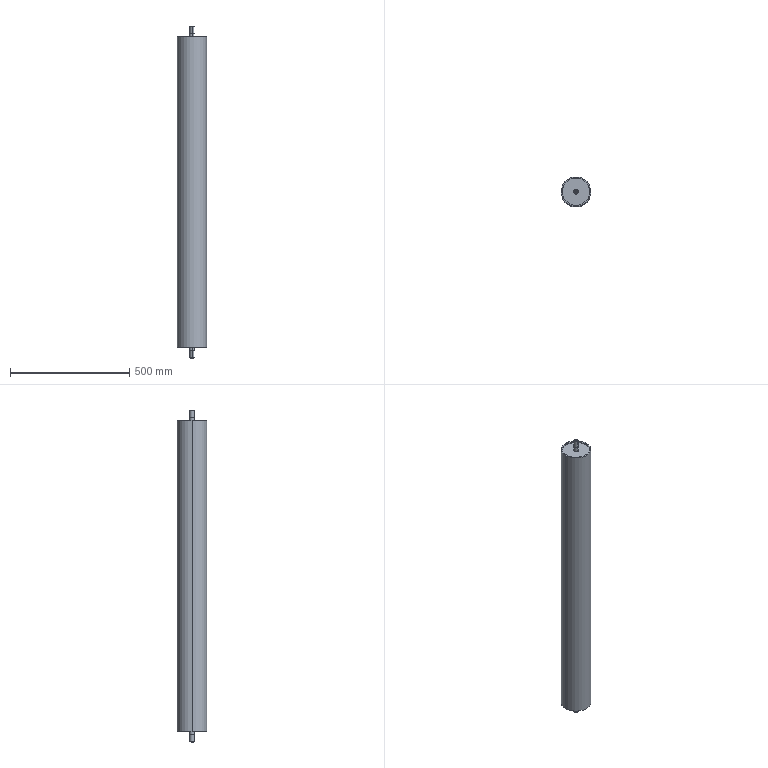Part | STEP file | Produce dryer-Driven part | 1 solid | 44 faces | box 124 x 124 x 1393 mm | volume 2869767 mm3 | cylinder 22 | cone 12 | plane 10 | commonest cylinder face diameters 20 x6 114.4 x6 5 x4 17 x4 124 x2
STEP:
#1=CARTESIAN_POINT('',(2.5,0.,-681.5));
#2=VERTEX_POINT('',#1);
#3=CARTESIAN_POINT('',(-2.5,0.,-681.5));
#4=VERTEX_POINT('',#3);
#5=CARTESIAN_POINT('',(0.,0.,-681.5));
#6=DIRECTION('',(0.,0.,-1.));
#7=DIRECTION('',(-1.,0.,0.));
#8=AXIS2_PLACEMENT_3D('',#5,#6,#7);
#9=CIRCLE('',#8,2.5);
#10=EDGE_CURVE('',#2,#4,#9,.T.);
#11=ORIENTED_EDGE('',*,*,#10,.F.);
#12=CARTESIAN_POINT('',(2.5,0.,-696.5));
#13=VERTEX_POINT('',#12);
#14=CARTESIAN_POINT('',(2.5,0.,-696.5));
#15=DIRECTION('',(0.,0.,-1.));
#16=VECTOR('',#15,1000.);
#17=LINE('',#14,#16);
#18=EDGE_CURVE('',#2,#13,#17,.T.);
#19=ORIENTED_EDGE('',*,*,#18,.T.);
#20=CARTESIAN_POINT('',(-2.5,0.,-696.5));
#21=VERTEX_POINT('',#20);
#22=CARTESIAN_POINT('',(0.,0.,-696.5));
#23=DIRECTION('',(0.,0.,-1.));
#24=DIRECTION('',(-1.,0.,0.));
#25=AXIS2_PLACEMENT_3D('',#22,#23,#24);
#26=CIRCLE('',#25,2.5);
#27=EDGE_CURVE('',#13,#21,#26,.T.);
#28=ORIENTED_EDGE('',*,*,#27,.T.);
#29=CARTESIAN_POINT('',(-2.5,0.,-696.5));
#30=DIRECTION('',(0.,0.,-1.));
#31=VECTOR('',#30,1000.);
#32=LINE('',#29,#31);
#33=EDGE_CURVE('',#4,#21,#32,.T.);
#34=ORIENTED_EDGE('',*,*,#33,.F.);
#35=EDGE_LOOP('',(#11,#19,#28,#34));
#36=FACE_OUTER_BOUND('',#35,.T.);
#37=CARTESIAN_POINT('',(0.,0.,-696.5));
#38=DIRECTION('',(0.,0.,-1.));
#39=DIRECTION('',(-1.,0.,0.));
#40=AXIS2_PLACEMENT_3D('',#37,#38,#39);
#41=CYLINDRICAL_SURFACE('',#40,2.5);
#42=ADVANCED_FACE('',(#36),#41,.F.);
#43=CARTESIAN_POINT('',(0.,0.,-679.998));
#44=VERTEX_POINT('',#43);
#45=CARTESIAN_POINT('',(-2.5,0.,-681.5));
#46=DIRECTION('',(-0.8572,0.,-0.515));
#47=VECTOR('',#46,1000.);
#48=LINE('',#45,#47);
#49=EDGE_CURVE('',#44,#4,#48,.T.);
#50=ORIENTED_EDGE('',*,*,#49,.F.);
#51=CARTESIAN_POINT('',(2.5,0.,-681.5));
#52=DIRECTION('',(0.8572,0.,-0.515));
#53=VECTOR('',#52,1000.);
#54=LINE('',#51,#53);
#55=EDGE_CURVE('',#44,#2,#54,.T.);
#56=ORIENTED_EDGE('',*,*,#55,.T.);
#57=ORIENTED_EDGE('',*,*,#10,.T.);
#58=EDGE_LOOP('',(#50,#56,#57));
#59=FACE_OUTER_BOUND('',#58,.T.);
#60=CARTESIAN_POINT('',(0.,0.,-681.5));
#61=DIRECTION('',(0.,0.,-1.));
#62=DIRECTION('',(-1.,0.,0.));
#63=AXIS2_PLACEMENT_3D('',#60,#61,#62);
#64=CONICAL_SURFACE('',#63,2.5,1.03);
#65=ADVANCED_FACE('',(#59),#64,.F.);
#66=CARTESIAN_POINT('',(0.,-10.,-665.));
#67=VERTEX_POINT('',#66);
#68=CARTESIAN_POINT('',(0.,10.,-665.));
#69=VERTEX_POINT('',#68);
#70=CARTESIAN_POINT('',(0.,0.,-665.));
#71=DIRECTION('',(0.,0.,1.));
#72=DIRECTION('',(0.,-1.,0.));
#73=AXIS2_PLACEMENT_3D('',#70,#71,#72);
#74=CIRCLE('',#73,10.);
#75=EDGE_CURVE('',#67,#69,#74,.T.);
#76=ORIENTED_EDGE('',*,*,#75,.T.);
#77=CARTESIAN_POINT('',(0.,10.,-645.5));
#78=VERTEX_POINT('',#77);
#79=CARTESIAN_POINT('',(0.,10.,-696.5));
#80=DIRECTION('',(0.,0.,1.));
#81=VECTOR('',#80,1000.);
#82=LINE('',#79,#81);
#83=EDGE_CURVE('',#69,#78,#82,.T.);
#84=ORIENTED_EDGE('',*,*,#83,.T.);
#85=CARTESIAN_POINT('',(0.,-10.,-645.5));
#86=VERTEX_POINT('',#85);
#87=CARTESIAN_POINT('',(0.,0.,-645.5));
#88=DIRECTION('',(0.,0.,-1.));
#89=DIRECTION('',(-1.,0.,0.));
#90=AXIS2_PLACEMENT_3D('',#87,#88,#89);
#91=CIRCLE('',#90,10.);
#92=EDGE_CURVE('',#78,#86,#91,.T.);
#93=ORIENTED_EDGE('',*,*,#92,.T.);
#94=CARTESIAN_POINT('',(0.,-10.,-696.5));
#95=DIRECTION('',(0.,0.,1.));
#96=VECTOR('',#95,1000.);
#97=LINE('',#94,#96);
#98=EDGE_CURVE('',#67,#86,#97,.T.);
#99=ORIENTED_EDGE('',*,*,#98,.F.);
#100=EDGE_LOOP('',(#76,#84,#93,#99));
#101=FACE_OUTER_BOUND('',#100,.T.);
#102=CARTESIAN_POINT('',(0.,0.,-696.5));
#103=DIRECTION('',(0.,0.,1.));
#104=DIRECTION('',(0.,-1.,0.));
#105=AXIS2_PLACEMENT_3D('',#102,#103,#104);
#106=CYLINDRICAL_SURFACE('',#105,10.);
#107=ADVANCED_FACE('',(#101),#106,.T.);
#108=CARTESIAN_POINT('',(0.,9.5,-665.5));
#109=VERTEX_POINT('',#108);
#110=CARTESIAN_POINT('',(0.,-9.5,-665.5));
#111=VERTEX_POINT('',#110);
#112=CARTESIAN_POINT('',(0.,0.,-665.5));
#113=DIRECTION('',(0.,0.,-1.));
#114=DIRECTION('',(0.,-1.,0.));
#115=AXIS2_PLACEMENT_3D('',#112,#113,#114);
#116=CIRCLE('',#115,9.5);
#117=EDGE_CURVE('',#109,#111,#116,.T.);
#118=ORIENTED_EDGE('',*,*,#117,.F.);
#119=CARTESIAN_POINT('',(0.,10.,-665.));
#120=DIRECTION('',(0.,0.7071,0.7071));
#121=VECTOR('',#120,1000.);
#122=LINE('',#119,#121);
#123=EDGE_CURVE('',#109,#69,#122,.T.);
#124=ORIENTED_EDGE('',*,*,#123,.T.);
#125=ORIENTED_EDGE('',*,*,#75,.F.);
#126=CARTESIAN_POINT('',(0.,-10.,-665.));
#127=DIRECTION('',(0.,-0.7071,0.7071));
#128=VECTOR('',#127,1000.);
#129=LINE('',#126,#128);
#130=EDGE_CURVE('',#111,#67,#129,.T.);
#131=ORIENTED_EDGE('',*,*,#130,.F.);
#132=EDGE_LOOP('',(#118,#124,#125,#131));
#133=FACE_OUTER_BOUND('',#132,.T.);
#134=CARTESIAN_POINT('',(0.,0.,-665.));
#135=DIRECTION('',(0.,0.,1.));
#136=DIRECTION('',(0.,-1.,0.));
#137=AXIS2_PLACEMENT_3D('',#134,#135,#136);
#138=CONICAL_SURFACE('',#137,10.,0.7854);
#139=ADVANCED_FACE('',(#133),#138,.T.);
#140=CARTESIAN_POINT('',(0.,-8.5,-696.));
#141=VERTEX_POINT('',#140);
#142=CARTESIAN_POINT('',(0.,8.5,-696.));
#143=VERTEX_POINT('',#142);
#144=CARTESIAN_POINT('',(0.,0.,-696.));
#145=DIRECTION('',(0.,0.,1.));
#146=DIRECTION('',(0.,-1.,0.));
#147=AXIS2_PLACEMENT_3D('',#144,#145,#146);
#148=CIRCLE('',#147,8.5);
#149=EDGE_CURVE('',#141,#143,#148,.T.);
#150=ORIENTED_EDGE('',*,*,#149,.T.);
#151=CARTESIAN_POINT('',(0.,8.5,-665.5));
#152=VERTEX_POINT('',#151);
#153=CARTESIAN_POINT('',(0.,8.5,-696.5));
#154=DIRECTION('',(0.,0.,1.));
#155=VECTOR('',#154,1000.);
#156=LINE('',#153,#155);
#157=EDGE_CURVE('',#143,#152,#156,.T.);
#158=ORIENTED_EDGE('',*,*,#157,.T.);
#159=CARTESIAN_POINT('',(0.,-8.5,-665.5));
#160=VERTEX_POINT('',#159);
#161=CARTESIAN_POINT('',(0.,0.,-665.5));
#162=DIRECTION('',(0.,0.,1.));
#163=DIRECTION('',(0.,-1.,0.));
#164=AXIS2_PLACEMENT_3D('',#161,#162,#163);
#165=CIRCLE('',#164,8.5);
#166=EDGE_CURVE('',#160,#152,#165,.T.);
#167=ORIENTED_EDGE('',*,*,#166,.F.);
#168=CARTESIAN_POINT('',(0.,-8.5,-696.5));
#169=DIRECTION('',(0.,0.,1.));
#170=VECTOR('',#169,1000.);
#171=LINE('',#168,#170);
#172=EDGE_CURVE('',#141,#160,#171,.T.);
#173=ORIENTED_EDGE('',*,*,#172,.F.);
#174=EDGE_LOOP('',(#150,#158,#167,#173));
#175=FACE_OUTER_BOUND('',#174,.T.);
#176=CARTESIAN_POINT('',(0.,0.,-696.5));
#177=DIRECTION('',(0.,0.,1.));
#178=DIRECTION('',(0.,-1.,0.));
#179=AXIS2_PLACEMENT_3D('',#176,#177,#178);
#180=CYLINDRICAL_SURFACE('',#179,8.5);
#181=ADVANCED_FACE('',(#175),#180,.T.);
#182=CARTESIAN_POINT('',(0.,8.,-696.5));
#183=VERTEX_POINT('',#182);
#184=CARTESIAN_POINT('',(0.,-8.,-696.5));
#185=VERTEX_POINT('',#184);
#186=CARTESIAN_POINT('',(0.,0.,-696.5));
#187=DIRECTION('',(0.,0.,-1.));
#188=DIRECTION('',(0.,-1.,0.));
#189=AXIS2_PLACEMENT_3D('',#186,#187,#188);
#190=CIRCLE('',#189,8.);
#191=EDGE_CURVE('',#183,#185,#190,.T.);
#192=ORIENTED_EDGE('',*,*,#191,.F.);
#193=CARTESIAN_POINT('',(0.,8.5,-696.));
#194=DIRECTION('',(0.,0.7071,0.7071));
#195=VECTOR('',#194,1000.);
#196=LINE('',#193,#195);
#197=EDGE_CURVE('',#183,#143,#196,.T.);
#198=ORIENTED_EDGE('',*,*,#197,.T.);
#199=ORIENTED_EDGE('',*,*,#149,.F.);
#200=CARTESIAN_POINT('',(0.,-8.5,-696.));
#201=DIRECTION('',(0.,-0.7071,0.7071));
#202=VECTOR('',#201,1000.);
#203=LINE('',#200,#202);
#204=EDGE_CURVE('',#185,#141,#203,.T.);
#205=ORIENTED_EDGE('',*,*,#204,.F.);
#206=EDGE_LOOP('',(#192,#198,#199,#205));
#207=FACE_OUTER_BOUND('',#206,.T.);
#208=CARTESIAN_POINT('',(0.,0.,-696.));
#209=DIRECTION('',(0.,0.,1.));
#210=DIRECTION('',(0.,-1.,0.));
#211=AXIS2_PLACEMENT_3D('',#208,#209,#210);
#212=CONICAL_SURFACE('',#211,8.5,0.7854);
#213=ADVANCED_FACE('',(#207),#212,.T.);
#214=CARTESIAN_POINT('',(-2.5,0.,681.5));
#215=VERTEX_POINT('',#214);
#216=CARTESIAN_POINT('',(2.5,0.,681.5));
#217=VERTEX_POINT('',#216);
#218=CARTESIAN_POINT('',(0.,0.,681.5));
#219=DIRECTION('',(0.,0.,1.));
#220=DIRECTION('',(1.,0.,0.));
#221=AXIS2_PLACEMENT_3D('',#218,#219,#220);
#222=CIRCLE('',#221,2.5);
#223=EDGE_CURVE('',#215,#217,#222,.T.);
#224=ORIENTED_EDGE('',*,*,#223,.F.);
#225=CARTESIAN_POINT('',(-2.5,0.,696.5));
#226=VERTEX_POINT('',#225);
#227=CARTESIAN_POINT('',(-2.5,0.,696.5));
#228=DIRECTION('',(0.,0.,1.));
#229=VECTOR('',#228,1000.);
#230=LINE('',#227,#229);
#231=EDGE_CURVE('',#215,#226,#230,.T.);
#232=ORIENTED_EDGE('',*,*,#231,.T.);
#233=CARTESIAN_POINT('',(2.5,0.,696.5));
#234=VERTEX_POINT('',#233);
#235=CARTESIAN_POINT('',(0.,0.,696.5));
#236=DIRECTION('',(0.,0.,1.));
#237=DIRECTION('',(1.,0.,0.));
#238=AXIS2_PLACEMENT_3D('',#235,#236,#237);
#239=CIRCLE('',#238,2.5);
#240=EDGE_CURVE('',#226,#234,#239,.T.);
#241=ORIENTED_EDGE('',*,*,#240,.T.);
#242=CARTESIAN_POINT('',(2.5,0.,696.5));
#243=DIRECTION('',(0.,0.,1.));
#244=VECTOR('',#243,1000.);
#245=LINE('',#242,#244);
#246=EDGE_CURVE('',#217,#234,#245,.T.);
#247=ORIENTED_EDGE('',*,*,#246,.F.);
#248=EDGE_LOOP('',(#224,#232,#241,#247));
#249=FACE_OUTER_BOUND('',#248,.T.);
#250=CARTESIAN_POINT('',(0.,0.,696.5));
#251=DIRECTION('',(0.,0.,1.));
#252=DIRECTION('',(1.,0.,0.));
#253=AXIS2_PLACEMENT_3D('',#250,#251,#252);
#254=CYLINDRICAL_SURFACE('',#253,2.5);
#255=ADVANCED_FACE('',(#249),#254,.F.);
#256=CARTESIAN_POINT('',(0.,0.,679.998));
#257=VERTEX_POINT('',#256);
#258=CARTESIAN_POINT('',(2.5,0.,681.5));
#259=DIRECTION('',(0.8572,0.,0.515));
#260=VECTOR('',#259,1000.);
#261=LINE('',#258,#260);
#262=EDGE_CURVE('',#257,#217,#261,.T.);
#263=ORIENTED_EDGE('',*,*,#262,.F.);
#264=CARTESIAN_POINT('',(-2.5,0.,681.5));
#265=DIRECTION('',(-0.8572,0.,0.515));
#266=VECTOR('',#265,1000.);
#267=LINE('',#264,#266);
#268=EDGE_CURVE('',#257,#215,#267,.T.);
#269=ORIENTED_EDGE('',*,*,#268,.T.);
#270=ORIENTED_EDGE('',*,*,#223,.T.);
#271=EDGE_LOOP('',(#263,#269,#270));
#272=FACE_OUTER_BOUND('',#271,.T.);
#273=CARTESIAN_POINT('',(0.,0.,681.5));
#274=DIRECTION('',(0.,0.,1.));
#275=DIRECTION('',(1.,0.,0.));
#276=AXIS2_PLACEMENT_3D('',#273,#274,#275);
#277=CONICAL_SURFACE('',#276,2.5,1.03);
#278=ADVANCED_FACE('',(#272),#277,.F.);
#279=CARTESIAN_POINT('',(0.,-9.5,665.5));
#280=VERTEX_POINT('',#279);
#281=CARTESIAN_POINT('',(0.,9.5,665.5));
#282=VERTEX_POINT('',#281);
#283=CARTESIAN_POINT('',(0.,0.,665.5));
#284=DIRECTION('',(0.,0.,1.));
#285=DIRECTION('',(0.,1.,0.));
#286=AXIS2_PLACEMENT_3D('',#283,#284,#285);
#287=CIRCLE('',#286,9.5);
#288=EDGE_CURVE('',#280,#282,#287,.T.);
#289=ORIENTED_EDGE('',*,*,#288,.F.);
#290=CARTESIAN_POINT('',(0.,-10.,665.));
#291=VERTEX_POINT('',#290);
#292=CARTESIAN_POINT('',(0.,-9.5,665.5));
#293=DIRECTION('',(0.,-0.7071,-0.7071));
#294=VECTOR('',#293,1000.);
#295=LINE('',#292,#294);
#296=EDGE_CURVE('',#280,#291,#295,.T.);
#297=ORIENTED_EDGE('',*,*,#296,.T.);
#298=CARTESIAN_POINT('',(0.,10.,665.));
#299=VERTEX_POINT('',#298);
#300=CARTESIAN_POINT('',(0.,0.,665.));
#301=DIRECTION('',(0.,0.,-1.));
#302=DIRECTION('',(0.,1.,0.));
#303=AXIS2_PLACEMENT_3D('',#300,#301,#302);
#304=CIRCLE('',#303,10.);
#305=EDGE_CURVE('',#299,#291,#304,.T.);
#306=ORIENTED_EDGE('',*,*,#305,.F.);
#307=CARTESIAN_POINT('',(0.,9.5,665.5));
#308=DIRECTION('',(0.,0.7071,-0.7071));
#309=VECTOR('',#308,1000.);
#310=LINE('',#307,#309);
#311=EDGE_CURVE('',#282,#299,#310,.T.);
#312=ORIENTED_EDGE('',*,*,#311,.F.);
#313=EDGE_LOOP('',(#289,#297,#306,#312));
#314=FACE_OUTER_BOUND('',#313,.T.);
#315=CARTESIAN_POINT('',(0.,0.,665.5));
#316=DIRECTION('',(0.,0.,-1.));
#317=DIRECTION('',(0.,1.,0.));
#318=AXIS2_PLACEMENT_3D('',#315,#316,#317);
#319=CONICAL_SURFACE('',#318,9.5,0.7854);
#320=ADVANCED_FACE('',(#314),#319,.T.);
#321=CARTESIAN_POINT('',(0.,-8.,696.5));
#322=VERTEX_POINT('',#321);
#323=CARTESIAN_POINT('',(0.,8.,696.5));
#324=VERTEX_POINT('',#323);
#325=CARTESIAN_POINT('',(0.,0.,696.5));
#326=DIRECTION('',(0.,0.,1.));
#327=DIRECTION('',(0.,1.,0.));
#328=AXIS2_PLACEMENT_3D('',#325,#326,#327);
#329=CIRCLE('',#328,8.);
#330=EDGE_CURVE('',#322,#324,#329,.T.);
#331=ORIENTED_EDGE('',*,*,#330,.F.);
#332=CARTESIAN_POINT('',(0.,-8.5,696.));
#333=VERTEX_POINT('',#332);
#334=CARTESIAN_POINT('',(0.,-8.,696.5));
#335=DIRECTION('',(0.,-0.7071,-0.7071));
#336=VECTOR('',#335,1000.);
#337=LINE('',#334,#336);
#338=EDGE_CURVE('',#322,#333,#337,.T.);
#339=ORIENTED_EDGE('',*,*,#338,.T.);
#340=CARTESIAN_POINT('',(0.,8.5,696.));
#341=VERTEX_POINT('',#340);
#342=CARTESIAN_POINT('',(0.,0.,696.));
#343=DIRECTION('',(0.,0.,-1.));
#344=DIRECTION('',(0.,1.,0.));
#345=AXIS2_PLACEMENT_3D('',#342,#343,#344);
#346=CIRCLE('',#345,8.5);
#347=EDGE_CURVE('',#341,#333,#346,.T.);
#348=ORIENTED_EDGE('',*,*,#347,.F.);
#349=CARTESIAN_POINT('',(0.,8.,696.5));
#350=DIRECTION('',(0.,0.7071,-0.7071));
#351=VECTOR('',#350,1000.);
#352=LINE('',#349,#351);
#353=EDGE_CURVE('',#324,#341,#352,.T.);
#354=ORIENTED_EDGE('',*,*,#353,.F.);
#355=EDGE_LOOP('',(#331,#339,#348,#354));
#356=FACE_OUTER_BOUND('',#355,.T.);
#357=CARTESIAN_POINT('',(0.,0.,696.5));
#358=DIRECTION('',(0.,0.,-1.));
#359=DIRECTION('',(0.,1.,0.));
#360=AXIS2_PLACEMENT_3D('',#357,#358,#359);
#361=CONICAL_SURFACE('',#360,8.,0.7854);
#362=ADVANCED_FACE('',(#356),#361,.T.);
#363=CARTESIAN_POINT('',(0.,10.,645.5));
#364=VERTEX_POINT('',#363);
#365=CARTESIAN_POINT('',(0.,-10.,645.5));
#366=VERTEX_POINT('',#365);
#367=CARTESIAN_POINT('',(0.,0.,645.5));
#368=DIRECTION('',(0.,0.,-1.));
#369=DIRECTION('',(1.,0.,0.));
#370=AXIS2_PLACEMENT_3D('',#367,#368,#369);
#371=CIRCLE('',#370,10.);
#372=EDGE_CURVE('',#364,#366,#371,.T.);
#373=ORIENTED_EDGE('',*,*,#372,.F.);
#374=CARTESIAN_POINT('',(0.,10.,-696.5));
#375=DIRECTION('',(0.,0.,1.));
#376=VECTOR('',#375,1000.);
#377=LINE('',#374,#376);
#378=EDGE_CURVE('',#364,#299,#377,.T.);
#379=ORIENTED_EDGE('',*,*,#378,.T.);
#380=ORIENTED_EDGE('',*,*,#305,.T.);
#381=CARTESIAN_POINT('',(0.,-10.,-696.5));
#382=DIRECTION('',(0.,0.,1.));
#383=VECTOR('',#382,1000.);
#384=LINE('',#381,#383);
#385=EDGE_CURVE('',#366,#291,#384,.T.);
#386=ORIENTED_EDGE('',*,*,#385,.F.);
#387=EDGE_LOOP('',(#373,#379,#380,#386));
#388=FACE_OUTER_BOUND('',#387,.T.);
#389=CARTESIAN_POINT('',(0.,0.,-696.5));
#390=DIRECTION('',(0.,0.,1.));
#391=DIRECTION('',(0.,-1.,0.));
#392=AXIS2_PLACEMENT_3D('',#389,#390,#391);
#393=CYLINDRICAL_SURFACE('',#392,10.);
#394=ADVANCED_FACE('',(#388),#393,.T.);
#395=CARTESIAN_POINT('',(0.,-8.5,665.5));
#396=VERTEX_POINT('',#395);
#397=CARTESIAN_POINT('',(0.,8.5,665.5));
#398=VERTEX_POINT('',#397);
#399=CARTESIAN_POINT('',(0.,0.,665.5));
#400=DIRECTION('',(0.,0.,1.));
#401=DIRECTION('',(0.,-1.,0.));
#402=AXIS2_PLACEMENT_3D('',#399,#400,#401);
#403=CIRCLE('',#402,8.5);
#404=EDGE_CURVE('',#396,#398,#403,.T.);
#405=ORIENTED_EDGE('',*,*,#404,.T.);
#406=CARTESIAN_POINT('',(0.,8.5,-696.5));
#407=DIRECTION('',(0.,0.,1.));
#408=VECTOR('',#407,1000.);
#409=LINE('',#406,#408);
#410=EDGE_CURVE('',#398,#341,#409,.T.);
#411=ORIENTED_EDGE('',*,*,#410,.T.);
#412=ORIENTED_EDGE('',*,*,#347,.T.);
#413=CARTESIAN_POINT('',(0.,-8.5,-696.5));
#414=DIRECTION('',(0.,0.,1.));
#415=VECTOR('',#414,1000.);
#416=LINE('',#413,#415);
#417=EDGE_CURVE('',#396,#333,#416,.T.);
#418=ORIENTED_EDGE('',*,*,#417,.F.);
#419=EDGE_LOOP('',(#405,#411,#412,#418));
#420=FACE_OUTER_BOUND('',#419,.T.);
#421=CARTESIAN_POINT('',(0.,0.,-696.5));
#422=DIRECTION('',(0.,0.,1.));
#423=DIRECTION('',(0.,-1.,0.));
#424=AXIS2_PLACEMENT_3D('',#421,#422,#423);
#425=CYLINDRICAL_SURFACE('',#424,8.5);
#426=ADVANCED_FACE('',(#420),#425,.T.);
#427=CARTESIAN_POINT('',(-57.2,0.,650.5));
#428=VERTEX_POINT('',#427);
#429=CARTESIAN_POINT('',(57.2,0.,650.5));
#430=VERTEX_POINT('',#429);
#431=CARTESIAN_POINT('',(0.,0.,650.5));
#432=DIRECTION('',(0.,0.,1.));
#433=DIRECTION('',(1.,0.,0.));
#434=AXIS2_PLACEMENT_3D('',#431,#432,#433);
#435=CIRCLE('',#434,57.2);
#436=EDGE_CURVE('',#428,#430,#435,.T.);
#437=ORIENTED_EDGE('',*,*,#436,.T.);
#438=CARTESIAN_POINT('',(57.2,0.,645.5));
#439=VERTEX_POINT('',#438);
#440=CARTESIAN_POINT('',(57.2,0.,650.5));
#441=DIRECTION('',(0.,0.,-1.));
#442=VECTOR('',#441,1000.);
#443=LINE('',#440,#442);
#444=EDGE_CURVE('',#430,#439,#443,.T.);
#445=ORIENTED_EDGE('',*,*,#444,.T.);
#446=CARTESIAN_POINT('',(-57.2,0.,645.5));
#447=VERTEX_POINT('',#446);
#448=CARTESIAN_POINT('',(0.,0.,645.5));
#449=DIRECTION('',(0.,0.,1.));
#450=DIRECTION('',(1.,0.,0.));
#451=AXIS2_PLACEMENT_3D('',#448,#449,#450);
#452=CIRCLE('',#451,57.2);
#453=EDGE_CURVE('',#447,#439,#452,.T.);
#454=ORIENTED_EDGE('',*,*,#453,.F.);
#455=CARTESIAN_POINT('',(-57.2,0.,650.5));
#456=DIRECTION('',(0.,0.,-1.));
#457=VECTOR('',#456,1000.);
#458=LINE('',#455,#457);
#459=EDGE_CURVE('',#428,#447,#458,.T.);
#460=ORIENTED_EDGE('',*,*,#459,.F.);
#461=EDGE_LOOP('',(#437,#445,#454,#460));
#462=FACE_OUTER_BOUND('',#461,.T.);
#463=CARTESIAN_POINT('',(0.,0.,650.5));
#464=DIRECTION('',(0.,0.,-1.));
#465=DIRECTION('',(-1.,0.,0.));
#466=AXIS2_PLACEMENT_3D('',#463,#464,#465);
#467=CYLINDRICAL_SURFACE('',#466,57.2);
#468=ADVANCED_FACE('',(#462),#467,.F.);
#469=CARTESIAN_POINT('',(62.,0.,650.5));
#470=VERTEX_POINT('',#469);
#471=CARTESIAN_POINT('',(-62.,0.,650.5));
#472=VERTEX_POINT('',#471);
#473=CARTESIAN_POINT('',(0.,0.,650.5));
#474=DIRECTION('',(0.,0.,1.));
#475=DIRECTION('',(1.,0.,0.));
#476=AXIS2_PLACEMENT_3D('',#473,#474,#475);
#477=CIRCLE('',#476,62.);
#478=EDGE_CURVE('',#470,#472,#477,.T.);
#479=ORIENTED_EDGE('',*,*,#478,.F.);
#480=CARTESIAN_POINT('',(62.,0.,-650.5));
#481=VERTEX_POINT('',#480);
#482=CARTESIAN_POINT('',(62.,0.,650.5));
#483=DIRECTION('',(0.,0.,-1.));
#484=VECTOR('',#483,1000.);
#485=LINE('',#482,#484);
#486=EDGE_CURVE('',#470,#481,#485,.T.);
#487=ORIENTED_EDGE('',*,*,#486,.T.);
#488=CARTESIAN_POINT('',(-62.,0.,-650.5));
#489=VERTEX_POINT('',#488);
#490=CARTESIAN_POINT('',(0.,0.,-650.5));
#491=DIRECTION('',(0.,0.,1.));
#492=DIRECTION('',(1.,0.,0.));
#493=AXIS2_PLACEMENT_3D('',#490,#491,#492);
#494=CIRCLE('',#493,62.);
#495=EDGE_CURVE('',#481,#489,#494,.T.);
#496=ORIENTED_EDGE('',*,*,#495,.T.);
#497=CARTESIAN_POINT('',(-62.,0.,650.5));
#498=DIRECTION('',(0.,0.,-1.));
#499=VECTOR('',#498,1000.);
#500=LINE('',#497,#499);
#501=EDGE_CURVE('',#472,#489,#500,.T.);
#502=ORIENTED_EDGE('',*,*,#501,.F.);
#503=EDGE_LOOP('',(#479,#487,#496,#502));
#504=FACE_OUTER_BOUND('',#503,.T.);
#505=CARTESIAN_POINT('',(0.,0.,650.5));
#506=DIRECTION('',(0.,0.,-1.));
#507=DIRECTION('',(-1.,0.,0.));
#508=AXIS2_PLACEMENT_3D('',#505,#506,#507);
#509=CYLINDRICAL_SURFACE('',#508,62.);
#510=ADVANCED_FACE('',(#504),#509,.T.);
#511=CARTESIAN_POINT('',(57.2,0.,-645.5));
#512=VERTEX_POINT('',#511);
#513=CARTESIAN_POINT('',(-57.2,0.,-645.5));
#514=VERTEX_POINT('',#513);
#515=CARTESIAN_POINT('',(0.,0.,-645.5));
#516=DIRECTION('',(0.,0.,-1.));
#517=DIRECTION('',(-1.,0.,0.));
#518=AXIS2_PLACEMENT_3D('',#515,#516,#517);
#519=CIRCLE('',#518,57.2);
#520=EDGE_CURVE('',#512,#514,#519,.T.);
#521=ORIENTED_EDGE('',*,*,#520,.F.);
#522=CARTESIAN_POINT('',(57.2,0.,-650.5));
#523=VERTEX_POINT('',#522);
#524=CARTESIAN_POINT('',(57.2,0.,650.5));
#525=DIRECTION('',(0.,0.,-1.));
#526=VECTOR('',#525,1000.);
#527=LINE('',#524,#526);
#528=EDGE_CURVE('',#512,#523,#527,.T.);
#529=ORIENTED_EDGE('',*,*,#528,.T.);
#530=CARTESIAN_POINT('',(-57.2,0.,-650.5));
#531=VERTEX_POINT('',#530);
#532=CARTESIAN_POINT('',(0.,0.,-650.5));
#533=DIRECTION('',(0.,0.,1.));
#534=DIRECTION('',(1.,0.,0.));
#535=AXIS2_PLACEMENT_3D('',#532,#533,#534);
#536=CIRCLE('',#535,57.2);
#537=EDGE_CURVE('',#531,#523,#536,.T.);
#538=ORIENTED_EDGE('',*,*,#537,.F.);
#539=CARTESIAN_POINT('',(-57.2,0.,650.5));
#540=DIRECTION('',(0.,0.,-1.));
#541=VECTOR('',#540,1000.);
#542=LINE('',#539,#541);
#543=EDGE_CURVE('',#514,#531,#542,.T.);
#544=ORIENTED_EDGE('',*,*,#543,.F.);
#545=EDGE_LOOP('',(#521,#529,#538,#544));
#546=FACE_OUTER_BOUND('',#545,.T.);
#547=CARTESIAN_POINT('',(0.,0.,650.5));
#548=DIRECTION('',(0.,0.,-1.));
#549=DIRECTION('',(-1.,0.,0.));
#550=AXIS2_PLACEMENT_3D('',#547,#548,#549);
#551=CYLINDRICAL_SURFACE('',#550,57.2);
#552=ADVANCED_FACE('',(#546),#551,.F.);
#553=ORIENTED_EDGE('',*,*,#528,.F.);
#554=CARTESIAN_POINT('',(0.,0.,-645.5));
#555=DIRECTION('',(0.,0.,-1.));
#556=DIRECTION('',(-1.,0.,0.));
#557=AXIS2_PLACEMENT_3D('',#554,#555,#556);
#558=CIRCLE('',#557,57.2);
#559=EDGE_CURVE('',#514,#512,#558,.T.);
#560=ORIENTED_EDGE('',*,*,#559,.F.);
#561=ORIENTED_EDGE('',*,*,#543,.T.);
#562=CARTESIAN_POINT('',(0.,0.,-650.5));
#563=DIRECTION('',(0.,0.,1.));
#564=DIRECTION('',(1.,0.,0.));
#565=AXIS2_PLACEMENT_3D('',#562,#563,#564);
#566=CIRCLE('',#565,57.2);
#567=EDGE_CURVE('',#523,#531,#566,.T.);
#568=ORIENTED_EDGE('',*,*,#567,.F.);
#569=EDGE_LOOP('',(#553,#560,#561,#568));
#570=FACE_OUTER_BOUND('',#569,.T.);
#571=CARTESIAN_POINT('',(0.,0.,650.5));
#572=DIRECTION('',(0.,0.,-1.));
#573=DIRECTION('',(-1.,0.,0.));
#574=AXIS2_PLACEMENT_3D('',#571,#572,#573);
#575=CYLINDRICAL_SURFACE('',#574,57.2);
#576=ADVANCED_FACE('',(#570),#575,.F.);
#577=CARTESIAN_POINT('',(0.,0.,650.5));
#578=DIRECTION('',(0.,0.,1.));
#579=DIRECTION('',(1.,0.,0.));
#580=AXIS2_PLACEMENT_3D('',#577,#578,#579);
#581=CIRCLE('',#580,62.);
#582=EDGE_CURVE('',#472,#470,#581,.T.);
#583=ORIENTED_EDGE('',*,*,#582,.T.);
#584=ORIENTED_EDGE('',*,*,#478,.T.);
#585=EDGE_LOOP('',(#583,#584));
#586=FACE_OUTER_BOUND('',#585,.T.);
#587=ORIENTED_EDGE('',*,*,#436,.F.);
#588=CARTESIAN_POINT('',(0.,0.,650.5));
#589=DIRECTION('',(0.,0.,1.));
#590=DIRECTION('',(1.,0.,0.));
#591=AXIS2_PLACEMENT_3D('',#588,#589,#590);
#592=CIRCLE('',#591,57.2);
#593=EDGE_CURVE('',#430,#428,#592,.T.);
#594=ORIENTED_EDGE('',*,*,#593,.F.);
#595=EDGE_LOOP('',(#587,#594));
#596=FACE_BOUND('',#595,.T.);
#597=CARTESIAN_POINT('',(0.,0.,650.5));
#598=DIRECTION('',(0.,0.,1.));
#599=DIRECTION('',(1.,0.,0.));
#600=AXIS2_PLACEMENT_3D('',#597,#598,#599);
#601=PLANE('',#600);
#602=ADVANCED_FACE('',(#586,#596),#601,.T.);
#603=CARTESIAN_POINT('',(0.,0.,-650.5));
#604=DIRECTION('',(0.,0.,1.));
#605=DIRECTION('',(1.,0.,0.));
#606=AXIS2_PLACEMENT_3D('',#603,#604,#605);
#607=CIRCLE('',#606,62.);
#608=EDGE_CURVE('',#489,#481,#607,.T.);
#609=ORIENTED_EDGE('',*,*,#608,.F.);
#610=ORIENTED_EDGE('',*,*,#495,.F.);
#611=EDGE_LOOP('',(#609,#610));
#612=FACE_OUTER_BOUND('',#611,.T.);
#613=ORIENTED_EDGE('',*,*,#537,.T.);
#614=ORIENTED_EDGE('',*,*,#567,.T.);
#615=EDGE_LOOP('',(#613,#614));
#616=FACE_BOUND('',#615,.T.);
#617=CARTESIAN_POINT('',(0.,0.,-650.5));
#618=DIRECTION('',(0.,0.,1.));
#619=DIRECTION('',(1.,0.,0.));
#620=AXIS2_PLACEMENT_3D('',#617,#618,#619);
#621=PLANE('',#620);
#622=ADVANCED_FACE('',(#612,#616),#621,.F.);
#623=ORIENTED_EDGE('',*,*,#486,.F.);
#624=ORIENTED_EDGE('',*,*,#582,.F.);
#625=ORIENTED_EDGE('',*,*,#501,.T.);
#626=ORIENTED_EDGE('',*,*,#608,.T.);
#627=EDGE_LOOP('',(#623,#624,#625,#626));
#628=FACE_OUTER_BOUND('',#627,.T.);
#629=CARTESIAN_POINT('',(0.,0.,650.5));
#630=DIRECTION('',(0.,0.,-1.));
#631=DIRECTION('',(-1.,0.,0.));
#632=AXIS2_PLACEMENT_3D('',#629,#630,#631);
#633=CYLINDRICAL_SURFACE('',#632,62.);
#634=ADVANCED_FACE('',(#628),#633,.T.);
#635=ORIENTED_EDGE('',*,*,#444,.F.);
#636=ORIENTED_EDGE('',*,*,#593,.T.);
#637=ORIENTED_EDGE('',*,*,#459,.T.);
#638=CARTESIAN_POINT('',(0.,0.,645.5));
#639=DIRECTION('',(0.,0.,1.));
#640=DIRECTION('',(1.,0.,0.));
#641=AXIS2_PLACEMENT_3D('',#638,#639,#640);
#642=CIRCLE('',#641,57.2);
#643=EDGE_CURVE('',#439,#447,#642,.T.);
#644=ORIENTED_EDGE('',*,*,#643,.F.);
#645=EDGE_LOOP('',(#635,#636,#637,#644));
#646=FACE_OUTER_BOUND('',#645,.T.);
#647=CARTESIAN_POINT('',(0.,0.,650.5));
#648=DIRECTION('',(0.,0.,-1.));
#649=DIRECTION('',(-1.,0.,0.));
#650=AXIS2_PLACEMENT_3D('',#647,#648,#649);
#651=CYLINDRICAL_SURFACE('',#650,57.2);
#652=ADVANCED_FACE('',(#646),#651,.F.);
#653=CARTESIAN_POINT('',(0.,0.,645.5));
#654=DIRECTION('',(0.,0.,-1.));
#655=DIRECTION('',(1.,0.,0.));
#656=AXIS2_PLACEMENT_3D('',#653,#654,#655);
#657=CIRCLE('',#656,10.);
#658=EDGE_CURVE('',#366,#364,#657,.T.);
#659=ORIENTED_EDGE('',*,*,#658,.T.);
#660=ORIENTED_EDGE('',*,*,#372,.T.);
#661=EDGE_LOOP('',(#659,#660));
#662=FACE_BOUND('',#661,.T.);
#663=ORIENTED_EDGE('',*,*,#453,.T.);
#664=ORIENTED_EDGE('',*,*,#643,.T.);
#665=EDGE_LOOP('',(#663,#664));
#666=FACE_OUTER_BOUND('',#665,.T.);
#667=CARTESIAN_POINT('',(0.,0.,645.5));
#668=DIRECTION('',(0.,0.,1.));
#669=DIRECTION('',(1.,0.,0.));
#670=AXIS2_PLACEMENT_3D('',#667,#668,#669);
#671=PLANE('',#670);
#672=ADVANCED_FACE('',(#662,#666),#671,.T.);
#673=CARTESIAN_POINT('',(0.,0.,696.5));
#674=DIRECTION('',(0.,0.,1.));
#675=DIRECTION('',(1.,0.,0.));
#676=AXIS2_PLACEMENT_3D('',#673,#674,#675);
#677=CIRCLE('',#676,2.5);
#678=EDGE_CURVE('',#234,#226,#677,.T.);
#679=ORIENTED_EDGE('',*,*,#678,.F.);
#680=ORIENTED_EDGE('',*,*,#240,.F.);
#681=EDGE_LOOP('',(#679,#680));
#682=FACE_BOUND('',#681,.T.);
#683=CARTESIAN_POINT('',(0.,0.,696.5));
#684=DIRECTION('',(0.,0.,1.));
#685=DIRECTION('',(0.,1.,0.));
#686=AXIS2_PLACEMENT_3D('',#683,#684,#685);
#687=CIRCLE('',#686,8.);
#688=EDGE_CURVE('',#324,#322,#687,.T.);
#689=ORIENTED_EDGE('',*,*,#688,.T.);
#690=ORIENTED_EDGE('',*,*,#330,.T.);
#691=EDGE_LOOP('',(#689,#690));
#692=FACE_OUTER_BOUND('',#691,.T.);
#693=CARTESIAN_POINT('',(0.,0.,696.5));
#694=DIRECTION('',(0.,0.,-1.));
#695=DIRECTION('',(0.,1.,0.));
#696=AXIS2_PLACEMENT_3D('',#693,#694,#695);
#697=PLANE('',#696);
#698=ADVANCED_FACE('',(#682,#692),#697,.F.);
#699=ORIENTED_EDGE('',*,*,#410,.F.);
#700=CARTESIAN_POINT('',(0.,0.,665.5));
#701=DIRECTION('',(0.,0.,1.));
#702=DIRECTION('',(0.,-1.,0.));
#703=AXIS2_PLACEMENT_3D('',#700,#701,#702);
#704=CIRCLE('',#703,8.5);
#705=EDGE_CURVE('',#398,#396,#704,.T.);
#706=ORIENTED_EDGE('',*,*,#705,.T.);
#707=ORIENTED_EDGE('',*,*,#417,.T.);
#708=CARTESIAN_POINT('',(0.,0.,696.));
#709=DIRECTION('',(0.,0.,-1.));
#710=DIRECTION('',(0.,1.,0.));
#711=AXIS2_PLACEMENT_3D('',#708,#709,#710);
#712=CIRCLE('',#711,8.5);
#713=EDGE_CURVE('',#333,#341,#712,.T.);
#714=ORIENTED_EDGE('',*,*,#713,.T.);
#715=EDGE_LOOP('',(#699,#706,#707,#714));
#716=FACE_OUTER_BOUND('',#715,.T.);
#717=CARTESIAN_POINT('',(0.,0.,-696.5));
#718=DIRECTION('',(0.,0.,1.));
#719=DIRECTION('',(0.,-1.,0.));
#720=AXIS2_PLACEMENT_3D('',#717,#718,#719);
#721=CYLINDRICAL_SURFACE('',#720,8.5);
#722=ADVANCED_FACE('',(#716),#721,.T.);
#723=CARTESIAN_POINT('',(0.,0.,665.5));
#724=DIRECTION('',(0.,0.,1.));
#725=DIRECTION('',(0.,1.,0.));
#726=AXIS2_PLACEMENT_3D('',#723,#724,#725);
#727=CIRCLE('',#726,9.5);
#728=EDGE_CURVE('',#282,#280,#727,.T.);
#729=ORIENTED_EDGE('',*,*,#728,.T.);
#730=ORIENTED_EDGE('',*,*,#288,.T.);
#731=EDGE_LOOP('',(#729,#730));
#732=FACE_OUTER_BOUND('',#731,.T.);
#733=ORIENTED_EDGE('',*,*,#404,.F.);
#734=ORIENTED_EDGE('',*,*,#705,.F.);
#735=EDGE_LOOP('',(#733,#734));
#736=FACE_BOUND('',#735,.T.);
#737=CARTESIAN_POINT('',(0.,8.5,665.5));
#738=DIRECTION('',(0.,0.,-1.));
#739=DIRECTION('',(0.,1.,0.));
#740=AXIS2_PLACEMENT_3D('',#737,#738,#739);
#741=PLANE('',#740);
#742=ADVANCED_FACE('',(#732,#736),#741,.F.);
#743=ORIENTED_EDGE('',*,*,#378,.F.);
#744=ORIENTED_EDGE('',*,*,#658,.F.);
#745=ORIENTED_EDGE('',*,*,#385,.T.);
#746=CARTESIAN_POINT('',(0.,0.,665.));
#747=DIRECTION('',(0.,0.,-1.));
#748=DIRECTION('',(0.,1.,0.));
#749=AXIS2_PLACEMENT_3D('',#746,#747,#748);
#750=CIRCLE('',#749,10.);
#751=EDGE_CURVE('',#291,#299,#750,.T.);
#752=ORIENTED_EDGE('',*,*,#751,.T.);
#753=EDGE_LOOP('',(#743,#744,#745,#752));
#754=FACE_OUTER_BOUND('',#753,.T.);
#755=CARTESIAN_POINT('',(0.,0.,-696.5));
#756=DIRECTION('',(0.,0.,1.));
#757=DIRECTION('',(0.,-1.,0.));
#758=AXIS2_PLACEMENT_3D('',#755,#756,#757);
#759=CYLINDRICAL_SURFACE('',#758,10.);
#760=ADVANCED_FACE('',(#754),#759,.T.);
#761=ORIENTED_EDGE('',*,*,#338,.F.);
#762=ORIENTED_EDGE('',*,*,#688,.F.);
#763=ORIENTED_EDGE('',*,*,#353,.T.);
#764=ORIENTED_EDGE('',*,*,#713,.F.);
#765=EDGE_LOOP('',(#761,#762,#763,#764));
#766=FACE_OUTER_BOUND('',#765,.T.);
#767=CARTESIAN_POINT('',(0.,0.,696.5));
#768=DIRECTION('',(0.,0.,-1.));
#769=DIRECTION('',(0.,1.,0.));
#770=AXIS2_PLACEMENT_3D('',#767,#768,#769);
#771=CONICAL_SURFACE('',#770,8.,0.7854);
#772=ADVANCED_FACE('',(#766),#771,.T.);
#773=ORIENTED_EDGE('',*,*,#296,.F.);
#774=ORIENTED_EDGE('',*,*,#728,.F.);
#775=ORIENTED_EDGE('',*,*,#311,.T.);
#776=ORIENTED_EDGE('',*,*,#751,.F.);
#777=EDGE_LOOP('',(#773,#774,#775,#776));
#778=FACE_OUTER_BOUND('',#777,.T.);
#779=CARTESIAN_POINT('',(0.,0.,665.5));
#780=DIRECTION('',(0.,0.,-1.));
#781=DIRECTION('',(0.,1.,0.));
#782=AXIS2_PLACEMENT_3D('',#779,#780,#781);
#783=CONICAL_SURFACE('',#782,9.5,0.7854);
#784=ADVANCED_FACE('',(#778),#783,.T.);
#785=ORIENTED_EDGE('',*,*,#268,.F.);
#786=ORIENTED_EDGE('',*,*,#262,.T.);
#787=CARTESIAN_POINT('',(0.,0.,681.5));
#788=DIRECTION('',(0.,0.,1.));
#789=DIRECTION('',(1.,0.,0.));
#790=AXIS2_PLACEMENT_3D('',#787,#788,#789);
#791=CIRCLE('',#790,2.5);
#792=EDGE_CURVE('',#217,#215,#791,.T.);
#793=ORIENTED_EDGE('',*,*,#792,.T.);
#794=EDGE_LOOP('',(#785,#786,#793));
#795=FACE_OUTER_BOUND('',#794,.T.);
#796=CARTESIAN_POINT('',(0.,0.,681.5));
#797=DIRECTION('',(0.,0.,1.));
#798=DIRECTION('',(1.,0.,0.));
#799=AXIS2_PLACEMENT_3D('',#796,#797,#798);
#800=CONICAL_SURFACE('',#799,2.5,1.03);
#801=ADVANCED_FACE('',(#795),#800,.F.);
#802=ORIENTED_EDGE('',*,*,#231,.F.);
#803=ORIENTED_EDGE('',*,*,#792,.F.);
#804=ORIENTED_EDGE('',*,*,#246,.T.);
#805=ORIENTED_EDGE('',*,*,#678,.T.);
#806=EDGE_LOOP('',(#802,#803,#804,#805));
#807=FACE_OUTER_BOUND('',#806,.T.);
#808=CARTESIAN_POINT('',(0.,0.,696.5));
#809=DIRECTION('',(0.,0.,1.));
#810=DIRECTION('',(1.,0.,0.));
#811=AXIS2_PLACEMENT_3D('',#808,#809,#810);
#812=CYLINDRICAL_SURFACE('',#811,2.5);
#813=ADVANCED_FACE('',(#807),#812,.F.);
#814=CARTESIAN_POINT('',(0.,0.,-645.5));
#815=DIRECTION('',(0.,0.,-1.));
#816=DIRECTION('',(-1.,0.,0.));
#817=AXIS2_PLACEMENT_3D('',#814,#815,#816);
#818=CIRCLE('',#817,10.);
#819=EDGE_CURVE('',#86,#78,#818,.T.);
#820=ORIENTED_EDGE('',*,*,#819,.F.);
#821=ORIENTED_EDGE('',*,*,#92,.F.);
#822=EDGE_LOOP('',(#820,#821));
#823=FACE_BOUND('',#822,.T.);
#824=ORIENTED_EDGE('',*,*,#559,.T.);
#825=ORIENTED_EDGE('',*,*,#520,.T.);
#826=EDGE_LOOP('',(#824,#825));
#827=FACE_OUTER_BOUND('',#826,.T.);
#828=CARTESIAN_POINT('',(0.,0.,-645.5));
#829=DIRECTION('',(0.,0.,-1.));
#830=DIRECTION('',(1.,0.,0.));
#831=AXIS2_PLACEMENT_3D('',#828,#829,#830);
#832=PLANE('',#831);
#833=ADVANCED_FACE('',(#823,#827),#832,.T.);
#834=CARTESIAN_POINT('',(0.,0.,-696.5));
#835=DIRECTION('',(0.,0.,-1.));
#836=DIRECTION('',(-1.,0.,0.));
#837=AXIS2_PLACEMENT_3D('',#834,#835,#836);
#838=CIRCLE('',#837,2.5);
#839=EDGE_CURVE('',#21,#13,#838,.T.);
#840=ORIENTED_EDGE('',*,*,#839,.F.);
#841=ORIENTED_EDGE('',*,*,#27,.F.);
#842=EDGE_LOOP('',(#840,#841));
#843=FACE_BOUND('',#842,.T.);
#844=CARTESIAN_POINT('',(0.,0.,-696.5));
#845=DIRECTION('',(0.,0.,-1.));
#846=DIRECTION('',(0.,-1.,0.));
#847=AXIS2_PLACEMENT_3D('',#844,#845,#846);
#848=CIRCLE('',#847,8.);
#849=EDGE_CURVE('',#185,#183,#848,.T.);
#850=ORIENTED_EDGE('',*,*,#849,.T.);
#851=ORIENTED_EDGE('',*,*,#191,.T.);
#852=EDGE_LOOP('',(#850,#851));
#853=FACE_OUTER_BOUND('',#852,.T.);
#854=CARTESIAN_POINT('',(0.,8.5,-696.5));
#855=DIRECTION('',(0.,0.,1.));
#856=DIRECTION('',(0.,-1.,0.));
#857=AXIS2_PLACEMENT_3D('',#854,#855,#856);
#858=PLANE('',#857);
#859=ADVANCED_FACE('',(#843,#853),#858,.F.);
#860=ORIENTED_EDGE('',*,*,#197,.F.);
#861=ORIENTED_EDGE('',*,*,#849,.F.);
#862=ORIENTED_EDGE('',*,*,#204,.T.);
#863=CARTESIAN_POINT('',(0.,0.,-696.));
#864=DIRECTION('',(0.,0.,1.));
#865=DIRECTION('',(0.,-1.,0.));
#866=AXIS2_PLACEMENT_3D('',#863,#864,#865);
#867=CIRCLE('',#866,8.5);
#868=EDGE_CURVE('',#143,#141,#867,.T.);
#869=ORIENTED_EDGE('',*,*,#868,.F.);
#870=EDGE_LOOP('',(#860,#861,#862,#869));
#871=FACE_OUTER_BOUND('',#870,.T.);
#872=CARTESIAN_POINT('',(0.,0.,-696.));
#873=DIRECTION('',(0.,0.,1.));
#874=DIRECTION('',(0.,-1.,0.));
#875=AXIS2_PLACEMENT_3D('',#872,#873,#874);
#876=CONICAL_SURFACE('',#875,8.5,0.7854);
#877=ADVANCED_FACE('',(#871),#876,.T.);
#878=ORIENTED_EDGE('',*,*,#157,.F.);
#879=ORIENTED_EDGE('',*,*,#868,.T.);
#880=ORIENTED_EDGE('',*,*,#172,.T.);
#881=CARTESIAN_POINT('',(0.,0.,-665.5));
#882=DIRECTION('',(0.,0.,1.));
#883=DIRECTION('',(0.,-1.,0.));
#884=AXIS2_PLACEMENT_3D('',#881,#882,#883);
#885=CIRCLE('',#884,8.5);
#886=EDGE_CURVE('',#152,#160,#885,.T.);
#887=ORIENTED_EDGE('',*,*,#886,.F.);
#888=EDGE_LOOP('',(#878,#879,#880,#887));
#889=FACE_OUTER_BOUND('',#888,.T.);
#890=CARTESIAN_POINT('',(0.,0.,-696.5));
#891=DIRECTION('',(0.,0.,1.));
#892=DIRECTION('',(0.,-1.,0.));
#893=AXIS2_PLACEMENT_3D('',#890,#891,#892);
#894=CYLINDRICAL_SURFACE('',#893,8.5);
#895=ADVANCED_FACE('',(#889),#894,.T.);
#896=CARTESIAN_POINT('',(0.,0.,-665.5));
#897=DIRECTION('',(0.,0.,-1.));
#898=DIRECTION('',(0.,-1.,0.));
#899=AXIS2_PLACEMENT_3D('',#896,#897,#898);
#900=CIRCLE('',#899,9.5);
#901=EDGE_CURVE('',#111,#109,#900,.T.);
#902=ORIENTED_EDGE('',*,*,#901,.T.);
#903=ORIENTED_EDGE('',*,*,#117,.T.);
#904=EDGE_LOOP('',(#902,#903));
#905=FACE_OUTER_BOUND('',#904,.T.);
#906=ORIENTED_EDGE('',*,*,#166,.T.);
#907=ORIENTED_EDGE('',*,*,#886,.T.);
#908=EDGE_LOOP('',(#906,#907));
#909=FACE_BOUND('',#908,.T.);
#910=CARTESIAN_POINT('',(0.,10.,-665.5));
#911=DIRECTION('',(0.,0.,1.));
#912=DIRECTION('',(0.,-1.,0.));
#913=AXIS2_PLACEMENT_3D('',#910,#911,#912);
#914=PLANE('',#913);
#915=ADVANCED_FACE('',(#905,#909),#914,.F.);
#916=ORIENTED_EDGE('',*,*,#123,.F.);
#917=ORIENTED_EDGE('',*,*,#901,.F.);
#918=ORIENTED_EDGE('',*,*,#130,.T.);
#919=CARTESIAN_POINT('',(0.,0.,-665.));
#920=DIRECTION('',(0.,0.,1.));
#921=DIRECTION('',(0.,-1.,0.));
#922=AXIS2_PLACEMENT_3D('',#919,#920,#921);
#923=CIRCLE('',#922,10.);
#924=EDGE_CURVE('',#69,#67,#923,.T.);
#925=ORIENTED_EDGE('',*,*,#924,.F.);
#926=EDGE_LOOP('',(#916,#917,#918,#925));
#927=FACE_OUTER_BOUND('',#926,.T.);
#928=CARTESIAN_POINT('',(0.,0.,-665.));
#929=DIRECTION('',(0.,0.,1.));
#930=DIRECTION('',(0.,-1.,0.));
#931=AXIS2_PLACEMENT_3D('',#928,#929,#930);
#932=CONICAL_SURFACE('',#931,10.,0.7854);
#933=ADVANCED_FACE('',(#927),#932,.T.);
#934=ORIENTED_EDGE('',*,*,#83,.F.);
#935=ORIENTED_EDGE('',*,*,#924,.T.);
#936=ORIENTED_EDGE('',*,*,#98,.T.);
#937=ORIENTED_EDGE('',*,*,#819,.T.);
#938=EDGE_LOOP('',(#934,#935,#936,#937));
#939=FACE_OUTER_BOUND('',#938,.T.);
#940=CARTESIAN_POINT('',(0.,0.,-696.5));
#941=DIRECTION('',(0.,0.,1.));
#942=DIRECTION('',(0.,-1.,0.));
#943=AXIS2_PLACEMENT_3D('',#940,#941,#942);
#944=CYLINDRICAL_SURFACE('',#943,10.);
#945=ADVANCED_FACE('',(#939),#944,.T.);
#946=ORIENTED_EDGE('',*,*,#55,.F.);
#947=ORIENTED_EDGE('',*,*,#49,.T.);
#948=CARTESIAN_POINT('',(0.,0.,-681.5));
#949=DIRECTION('',(0.,0.,-1.));
#950=DIRECTION('',(-1.,0.,0.));
#951=AXIS2_PLACEMENT_3D('',#948,#949,#950);
#952=CIRCLE('',#951,2.5);
#953=EDGE_CURVE('',#4,#2,#952,.T.);
#954=ORIENTED_EDGE('',*,*,#953,.T.);
#955=EDGE_LOOP('',(#946,#947,#954));
#956=FACE_OUTER_BOUND('',#955,.T.);
#957=CARTESIAN_POINT('',(0.,0.,-681.5));
#958=DIRECTION('',(0.,0.,-1.));
#959=DIRECTION('',(-1.,0.,0.));
#960=AXIS2_PLACEMENT_3D('',#957,#958,#959);
#961=CONICAL_SURFACE('',#960,2.5,1.03);
#962=ADVANCED_FACE('',(#956),#961,.F.);
#963=ORIENTED_EDGE('',*,*,#18,.F.);
#964=ORIENTED_EDGE('',*,*,#953,.F.);
#965=ORIENTED_EDGE('',*,*,#33,.T.);
#966=ORIENTED_EDGE('',*,*,#839,.T.);
#967=EDGE_LOOP('',(#963,#964,#965,#966));
#968=FACE_OUTER_BOUND('',#967,.T.);
#969=CARTESIAN_POINT('',(0.,0.,-696.5));
#970=DIRECTION('',(0.,0.,-1.));
#971=DIRECTION('',(-1.,0.,0.));
#972=AXIS2_PLACEMENT_3D('',#969,#970,#971);
#973=CYLINDRICAL_SURFACE('',#972,2.5);
#974=ADVANCED_FACE('',(#968),#973,.F.);
#975=CLOSED_SHELL('',(#42,#65,#107,#139,#181,#213,#255,#278,#320,#362,#394,#426,#468,#510,#552,#576,#602,#622,#634,#652,#672,#698,#722,#742,#760,#772,#784,#801,#813,#833,#859,#877,#895,#915,#933,#945,#962,#974));
#976=CARTESIAN_POINT('',(0.,10.,-640.5));
#977=VERTEX_POINT('',#976);
#978=CARTESIAN_POINT('',(0.,-10.,-640.5));
#979=VERTEX_POINT('',#978);
#980=CARTESIAN_POINT('',(0.,0.,-640.5));
#981=DIRECTION('',(0.,0.,-1.));
#982=DIRECTION('',(-1.,0.,0.));
#983=AXIS2_PLACEMENT_3D('',#980,#981,#982);
#984=CIRCLE('',#983,10.);
#985=EDGE_CURVE('',#977,#979,#984,.T.);
#986=ORIENTED_EDGE('',*,*,#985,.F.);
#987=CARTESIAN_POINT('',(0.,10.,640.5));
#988=VERTEX_POINT('',#987);
#989=CARTESIAN_POINT('',(0.,10.,-696.5));
#990=DIRECTION('',(0.,0.,1.));
#991=VECTOR('',#990,1000.);
#992=LINE('',#989,#991);
#993=EDGE_CURVE('',#977,#988,#992,.T.);
#994=ORIENTED_EDGE('',*,*,#993,.T.);
#995=CARTESIAN_POINT('',(0.,-10.,640.5));
#996=VERTEX_POINT('',#995);
#997=CARTESIAN_POINT('',(0.,0.,640.5));
#998=DIRECTION('',(0.,0.,-1.));
#999=DIRECTION('',(1.,0.,0.));
#1000=AXIS2_PLACEMENT_3D('',#997,#998,#999);
#1001=CIRCLE('',#1000,10.);
#1002=EDGE_CURVE('',#988,#996,#1001,.T.);
#1003=ORIENTED_EDGE('',*,*,#1002,.T.);
#1004=CARTESIAN_POINT('',(0.,-10.,-696.5));
#1005=DIRECTION('',(0.,0.,1.));
#1006=VECTOR('',#1005,1000.);
#1007=LINE('',#1004,#1006);
#1008=EDGE_CURVE('',#979,#996,#1007,.T.);
#1009=ORIENTED_EDGE('',*,*,#1008,.F.);
#1010=EDGE_LOOP('',(#986,#994,#1003,#1009));
#1011=FACE_OUTER_BOUND('',#1010,.T.);
#1012=CARTESIAN_POINT('',(0.,0.,-696.5));
#1013=DIRECTION('',(0.,0.,1.));
#1014=DIRECTION('',(0.,-1.,0.));
#1015=AXIS2_PLACEMENT_3D('',#1012,#1013,#1014);
#1016=CYLINDRICAL_SURFACE('',#1015,10.);
#1017=ADVANCED_FACE('',(#1011),#1016,.T.);
#1018=CARTESIAN_POINT('',(-57.2,0.,640.5));
#1019=VERTEX_POINT('',#1018);
#1020=CARTESIAN_POINT('',(57.2,0.,640.5));
#1021=VERTEX_POINT('',#1020);
#1022=CARTESIAN_POINT('',(0.,0.,640.5));
#1023=DIRECTION('',(0.,0.,1.));
#1024=DIRECTION('',(1.,0.,0.));
#1025=AXIS2_PLACEMENT_3D('',#1022,#1023,#1024);
#1026=CIRCLE('',#1025,57.2);
#1027=EDGE_CURVE('',#1019,#1021,#1026,.T.);
#1028=ORIENTED_EDGE('',*,*,#1027,.T.);
#1029=CARTESIAN_POINT('',(57.2,0.,-640.5));
#1030=VERTEX_POINT('',#1029);
#1031=CARTESIAN_POINT('',(57.2,0.,650.5));
#1032=DIRECTION('',(0.,0.,-1.));
#1033=VECTOR('',#1032,1000.);
#1034=LINE('',#1031,#1033);
#1035=EDGE_CURVE('',#1021,#1030,#1034,.T.);
#1036=ORIENTED_EDGE('',*,*,#1035,.T.);
#1037=CARTESIAN_POINT('',(-57.2,0.,-640.5));
#1038=VERTEX_POINT('',#1037);
#1039=CARTESIAN_POINT('',(0.,0.,-640.5));
#1040=DIRECTION('',(0.,0.,1.));
#1041=DIRECTION('',(1.,0.,0.));
#1042=AXIS2_PLACEMENT_3D('',#1039,#1040,#1041);
#1043=CIRCLE('',#1042,57.2);
#1044=EDGE_CURVE('',#1038,#1030,#1043,.T.);
#1045=ORIENTED_EDGE('',*,*,#1044,.F.);
#1046=CARTESIAN_POINT('',(-57.2,0.,650.5));
#1047=DIRECTION('',(0.,0.,-1.));
#1048=VECTOR('',#1047,1000.);
#1049=LINE('',#1046,#1048);
#1050=EDGE_CURVE('',#1019,#1038,#1049,.T.);
#1051=ORIENTED_EDGE('',*,*,#1050,.F.);
#1052=EDGE_LOOP('',(#1028,#1036,#1045,#1051));
#1053=FACE_OUTER_BOUND('',#1052,.T.);
#1054=CARTESIAN_POINT('',(0.,0.,650.5));
#1055=DIRECTION('',(0.,0.,-1.));
#1056=DIRECTION('',(-1.,0.,0.));
#1057=AXIS2_PLACEMENT_3D('',#1054,#1055,#1056);
#1058=CYLINDRICAL_SURFACE('',#1057,57.2);
#1059=ADVANCED_FACE('',(#1053),#1058,.F.);
#1060=CARTESIAN_POINT('',(0.,0.,-640.5));
#1061=DIRECTION('',(0.,0.,-1.));
#1062=DIRECTION('',(-1.,0.,0.));
#1063=AXIS2_PLACEMENT_3D('',#1060,#1061,#1062);
#1064=CIRCLE('',#1063,10.);
#1065=EDGE_CURVE('',#979,#977,#1064,.T.);
#1066=ORIENTED_EDGE('',*,*,#1065,.T.);
#1067=ORIENTED_EDGE('',*,*,#985,.T.);
#1068=EDGE_LOOP('',(#1066,#1067));
#1069=FACE_BOUND('',#1068,.T.);
#1070=ORIENTED_EDGE('',*,*,#1044,.T.);
#1071=CARTESIAN_POINT('',(0.,0.,-640.5));
#1072=DIRECTION('',(0.,0.,1.));
#1073=DIRECTION('',(1.,0.,0.));
#1074=AXIS2_PLACEMENT_3D('',#1071,#1072,#1073);
#1075=CIRCLE('',#1074,57.2);
#1076=EDGE_CURVE('',#1030,#1038,#1075,.T.);
#1077=ORIENTED_EDGE('',*,*,#1076,.T.);
#1078=EDGE_LOOP('',(#1070,#1077));
#1079=FACE_OUTER_BOUND('',#1078,.T.);
#1080=CARTESIAN_POINT('',(0.,0.,-640.5));
#1081=DIRECTION('',(0.,0.,-1.));
#1082=DIRECTION('',(1.,0.,0.));
#1083=AXIS2_PLACEMENT_3D('',#1080,#1081,#1082);
#1084=PLANE('',#1083);
#1085=ADVANCED_FACE('',(#1069,#1079),#1084,.F.);
#1086=ORIENTED_EDGE('',*,*,#1035,.F.);
#1087=CARTESIAN_POINT('',(0.,0.,640.5));
#1088=DIRECTION('',(0.,0.,1.));
#1089=DIRECTION('',(1.,0.,0.));
#1090=AXIS2_PLACEMENT_3D('',#1087,#1088,#1089);
#1091=CIRCLE('',#1090,57.2);
#1092=EDGE_CURVE('',#1021,#1019,#1091,.T.);
#1093=ORIENTED_EDGE('',*,*,#1092,.T.);
#1094=ORIENTED_EDGE('',*,*,#1050,.T.);
#1095=ORIENTED_EDGE('',*,*,#1076,.F.);
#1096=EDGE_LOOP('',(#1086,#1093,#1094,#1095));
#1097=FACE_OUTER_BOUND('',#1096,.T.);
#1098=CARTESIAN_POINT('',(0.,0.,650.5));
#1099=DIRECTION('',(0.,0.,-1.));
#1100=DIRECTION('',(-1.,0.,0.));
#1101=AXIS2_PLACEMENT_3D('',#1098,#1099,#1100);
#1102=CYLINDRICAL_SURFACE('',#1101,57.2);
#1103=ADVANCED_FACE('',(#1097),#1102,.F.);
#1104=CARTESIAN_POINT('',(0.,0.,640.5));
#1105=DIRECTION('',(0.,0.,-1.));
#1106=DIRECTION('',(1.,0.,0.));
#1107=AXIS2_PLACEMENT_3D('',#1104,#1105,#1106);
#1108=CIRCLE('',#1107,10.);
#1109=EDGE_CURVE('',#996,#988,#1108,.T.);
#1110=ORIENTED_EDGE('',*,*,#1109,.F.);
#1111=ORIENTED_EDGE('',*,*,#1002,.F.);
#1112=EDGE_LOOP('',(#1110,#1111));
#1113=FACE_BOUND('',#1112,.T.);
#1114=ORIENTED_EDGE('',*,*,#1027,.F.);
#1115=ORIENTED_EDGE('',*,*,#1092,.F.);
#1116=EDGE_LOOP('',(#1114,#1115));
#1117=FACE_OUTER_BOUND('',#1116,.T.);
#1118=CARTESIAN_POINT('',(0.,0.,640.5));
#1119=DIRECTION('',(0.,0.,1.));
#1120=DIRECTION('',(1.,0.,0.));
#1121=AXIS2_PLACEMENT_3D('',#1118,#1119,#1120);
#1122=PLANE('',#1121);
#1123=ADVANCED_FACE('',(#1113,#1117),#1122,.F.);
#1124=ORIENTED_EDGE('',*,*,#993,.F.);
#1125=ORIENTED_EDGE('',*,*,#1065,.F.);
#1126=ORIENTED_EDGE('',*,*,#1008,.T.);
#1127=ORIENTED_EDGE('',*,*,#1109,.T.);
#1128=EDGE_LOOP('',(#1124,#1125,#1126,#1127));
#1129=FACE_OUTER_BOUND('',#1128,.T.);
#1130=CARTESIAN_POINT('',(0.,0.,-696.5));
#1131=DIRECTION('',(0.,0.,1.));
#1132=DIRECTION('',(0.,-1.,0.));
#1133=AXIS2_PLACEMENT_3D('',#1130,#1131,#1132);
#1134=CYLINDRICAL_SURFACE('',#1133,10.);
#1135=ADVANCED_FACE('',(#1129),#1134,.T.);
#1136=CLOSED_SHELL('',(#1017,#1059,#1085,#1103,#1123,#1135));
#1137=ORIENTED_CLOSED_SHELL('',*,#1136,.F.);
#1138=BREP_WITH_VOIDS('',#975,(#1137));
#1139=CARTESIAN_POINT('',(0.,0.,0.));
#1140=DIRECTION('',(0.,0.,1.));
#1141=DIRECTION('',(1.,0.,0.));
#1142=AXIS2_PLACEMENT_3D('',#1139,#1140,#1141);
#1143=(LENGTH_UNIT()NAMED_UNIT(*)SI_UNIT(.MILLI.,.METRE.));
#1144=UNCERTAINTY_MEASURE_WITH_UNIT(LENGTH_MEASURE(0.00001),#1143,'','');
#1145=(NAMED_UNIT(*)PLANE_ANGLE_UNIT()SI_UNIT($,.RADIAN.));
#1146=(NAMED_UNIT(*)SI_UNIT($,.STERADIAN.)SOLID_ANGLE_UNIT());
#1147=(GEOMETRIC_REPRESENTATION_CONTEXT(3)GLOBAL_UNCERTAINTY_ASSIGNED_CONTEXT((#1144))GLOBAL_UNIT_ASSIGNED_CONTEXT((#1143,#1145,#1146))REPRESENTATION_CONTEXT('',''));
#1148=ADVANCED_BREP_SHAPE_REPRESENTATION('',(#1138,#1142),#1147);